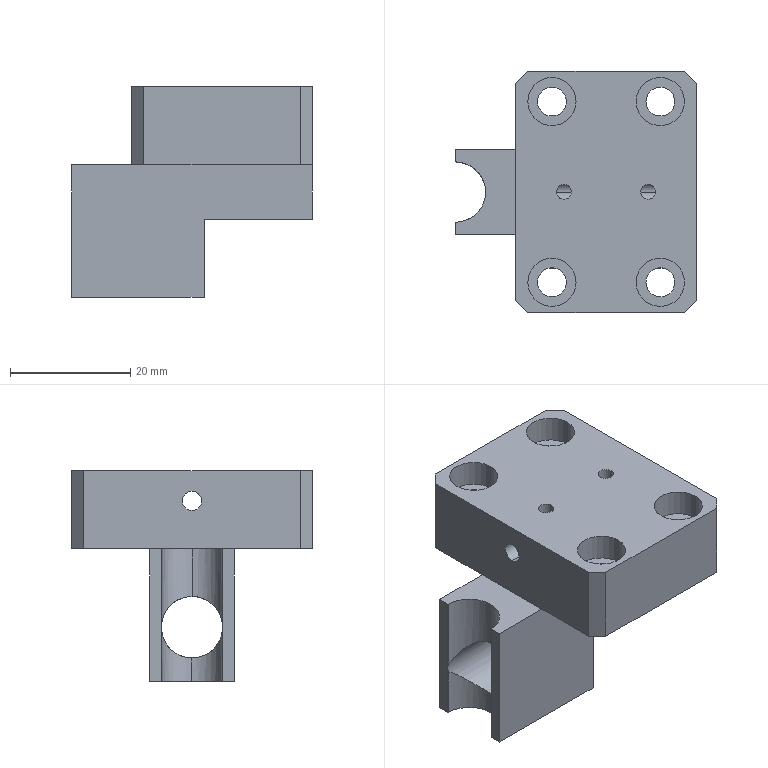Part | STEP file | PN_0001 | 1 solid | 57 faces | box 40 x 40 x 35 mm | volume 19874 mm3 | cylinder 29 | plane 28 | commonest cylinder face diameters 4.8 x8 8 x8 2.5 x4 10 x4 3.2 x2 10.2 x2